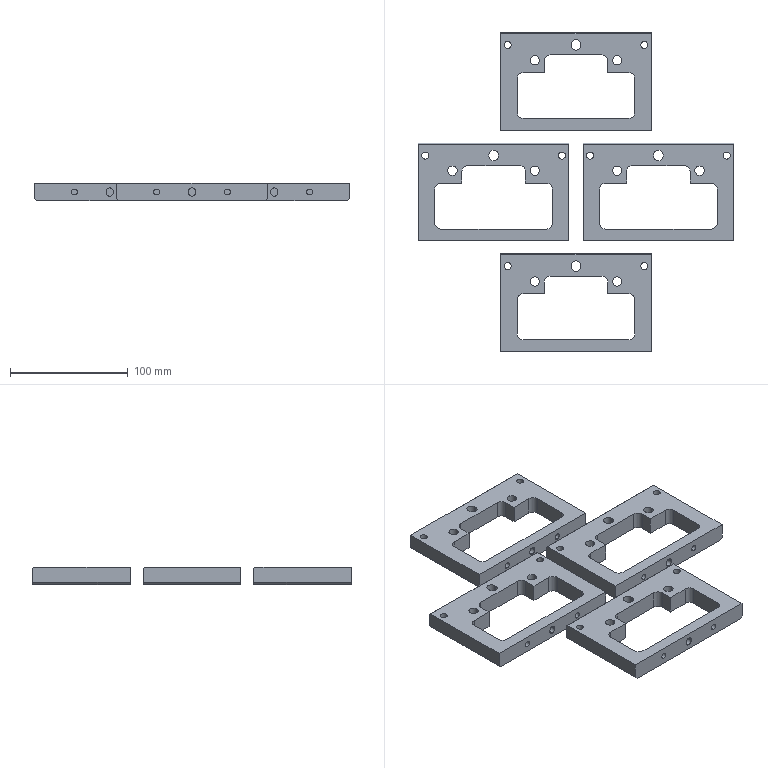Part | 4 solids | 180 faces | box 268 x 271 x 15 mm | volume 339599 mm3 | cylinder 92 | plane 88 | commonest cylinder face diameters 6 x28 8 x24 10 x24 5 x16